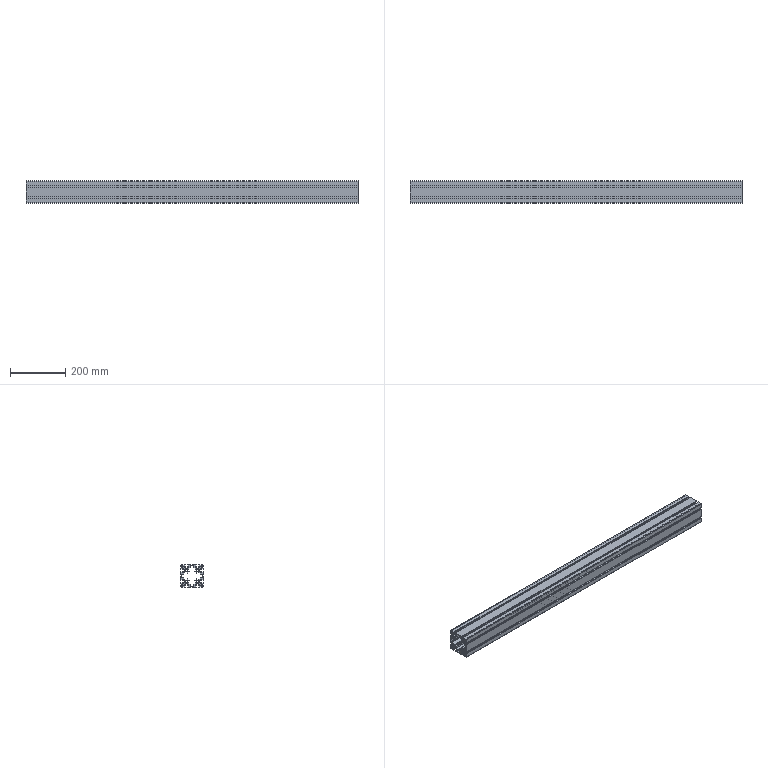Part | SolidWorks | features ICE 1, WeldMemberFeat 1, WeldmentFeature 1 | 1 solid | 174 faces | box 1200 x 80 x 80 mm | volume 2746825 mm3 | plane 146 | cylinder 28 | commonest cylinder face diameters 2 x8 6 x8 6.8 x8 3 x4